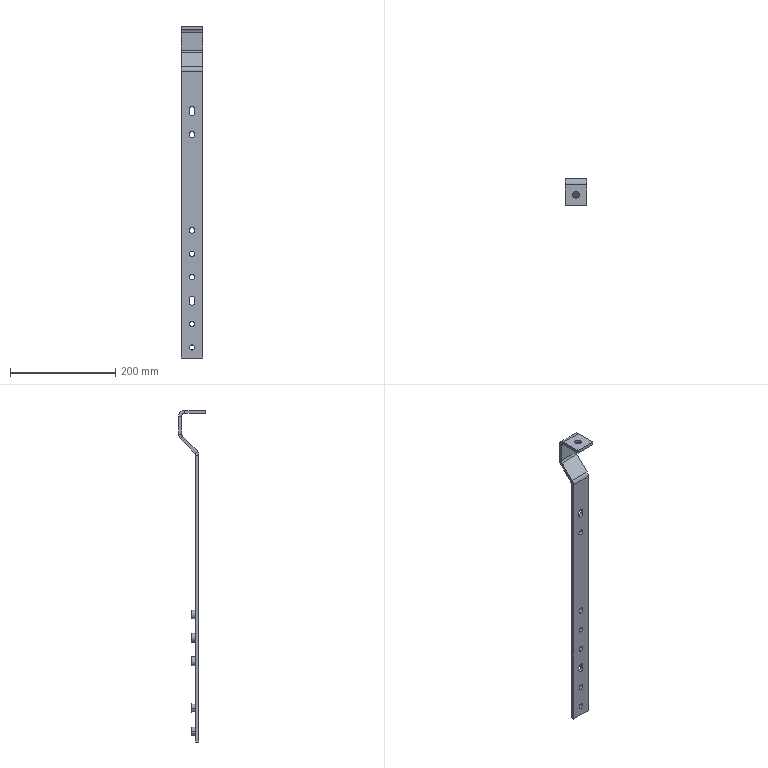Part | STEP file | 64805991 | 1 solid | 67 faces | box 40 x 51 x 631 mm | volume 163842 mm3 | cylinder 34 | plane 33 | commonest cylinder face diameters 16.5 x10 10 x8 11 x8 12 x3 24 x3 13 x2